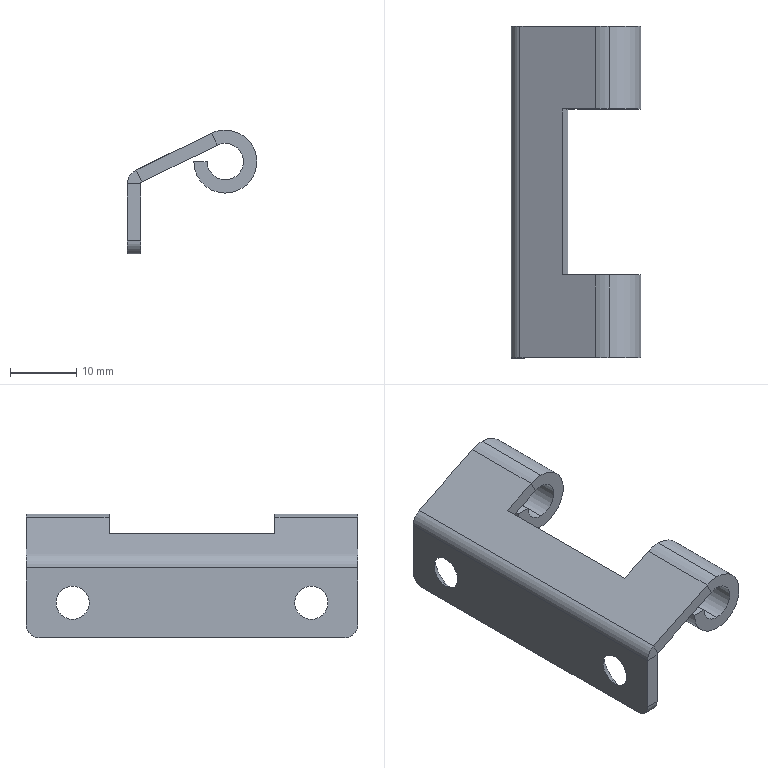Part | SolidWorks | features Cut 2, Chamfer 1, Fillet 1, FlatPattern 1, SMBaseFlange 1, SheetMetal 1 | 1 solid | 40 faces | box 19.5 x 50 x 18.659 mm | volume 2993 mm3 | plane 20 | cylinder 16 | cone 4 | commonest cylinder face diameters 5.5 x6 9.5 x6 4 x2 0.6 x1 4.6 x1
STEP:
#1=CARTESIAN_POINT('',(0.,43.,7.8));
#2=VERTEX_POINT('',#1);
#3=CARTESIAN_POINT('',(0.,43.,2.8));
#4=VERTEX_POINT('',#3);
#5=CARTESIAN_POINT('',(0.,43.,5.3));
#6=DIRECTION('',(1.,0.,0.));
#7=DIRECTION('',(0.,0.,-1.));
#8=AXIS2_PLACEMENT_3D('',#5,#6,#7);
#9=CIRCLE('',#8,2.5);
#10=EDGE_CURVE('',#2,#4,#9,.T.);
#11=ORIENTED_EDGE('',*,*,#10,.F.);
#12=CARTESIAN_POINT('',(2.,43.,9.8));
#13=VERTEX_POINT('',#12);
#14=CARTESIAN_POINT('',(0.,43.,7.8));
#15=DIRECTION('',(0.7071,0.,0.7071));
#16=VECTOR('',#15,1000.);
#17=LINE('',#14,#16);
#18=EDGE_CURVE('',#2,#13,#17,.T.);
#19=ORIENTED_EDGE('',*,*,#18,.T.);
#20=CARTESIAN_POINT('',(2.,43.,0.8));
#21=VERTEX_POINT('',#20);
#22=CARTESIAN_POINT('',(2.,43.,5.3));
#23=DIRECTION('',(-1.,0.,0.));
#24=DIRECTION('',(0.,0.,-1.));
#25=AXIS2_PLACEMENT_3D('',#22,#23,#24);
#26=CIRCLE('',#25,4.5);
#27=EDGE_CURVE('',#21,#13,#26,.T.);
#28=ORIENTED_EDGE('',*,*,#27,.F.);
#29=CARTESIAN_POINT('',(0.,43.,2.8));
#30=DIRECTION('',(0.7071,0.,-0.7071));
#31=VECTOR('',#30,1000.);
#32=LINE('',#29,#31);
#33=EDGE_CURVE('',#4,#21,#32,.T.);
#34=ORIENTED_EDGE('',*,*,#33,.F.);
#35=EDGE_LOOP('',(#11,#19,#28,#34));
#36=FACE_OUTER_BOUND('',#35,.T.);
#37=CARTESIAN_POINT('',(0.,43.,5.3));
#38=DIRECTION('',(1.,0.,0.));
#39=DIRECTION('',(0.,0.,-1.));
#40=AXIS2_PLACEMENT_3D('',#37,#38,#39);
#41=CONICAL_SURFACE('',#40,2.5,0.7854);
#42=ADVANCED_FACE('',(#36),#41,.F.);
#43=CARTESIAN_POINT('',(0.,7.,7.8));
#44=VERTEX_POINT('',#43);
#45=CARTESIAN_POINT('',(0.,7.,2.8));
#46=VERTEX_POINT('',#45);
#47=CARTESIAN_POINT('',(0.,7.,5.3));
#48=DIRECTION('',(1.,0.,0.));
#49=DIRECTION('',(0.,0.,-1.));
#50=AXIS2_PLACEMENT_3D('',#47,#48,#49);
#51=CIRCLE('',#50,2.5);
#52=EDGE_CURVE('',#44,#46,#51,.T.);
#53=ORIENTED_EDGE('',*,*,#52,.F.);
#54=CARTESIAN_POINT('',(2.,7.,9.8));
#55=VERTEX_POINT('',#54);
#56=CARTESIAN_POINT('',(0.,7.,7.8));
#57=DIRECTION('',(0.7071,0.,0.7071));
#58=VECTOR('',#57,1000.);
#59=LINE('',#56,#58);
#60=EDGE_CURVE('',#44,#55,#59,.T.);
#61=ORIENTED_EDGE('',*,*,#60,.T.);
#62=CARTESIAN_POINT('',(2.,7.,0.8));
#63=VERTEX_POINT('',#62);
#64=CARTESIAN_POINT('',(2.,7.,5.3));
#65=DIRECTION('',(-1.,0.,0.));
#66=DIRECTION('',(0.,0.,-1.));
#67=AXIS2_PLACEMENT_3D('',#64,#65,#66);
#68=CIRCLE('',#67,4.5);
#69=EDGE_CURVE('',#63,#55,#68,.T.);
#70=ORIENTED_EDGE('',*,*,#69,.F.);
#71=CARTESIAN_POINT('',(0.,7.,2.8));
#72=DIRECTION('',(0.7071,0.,-0.7071));
#73=VECTOR('',#72,1000.);
#74=LINE('',#71,#73);
#75=EDGE_CURVE('',#46,#63,#74,.T.);
#76=ORIENTED_EDGE('',*,*,#75,.F.);
#77=EDGE_LOOP('',(#53,#61,#70,#76));
#78=FACE_OUTER_BOUND('',#77,.T.);
#79=CARTESIAN_POINT('',(0.,7.,5.3));
#80=DIRECTION('',(1.,0.,0.));
#81=DIRECTION('',(0.,0.,-1.));
#82=AXIS2_PLACEMENT_3D('',#79,#80,#81);
#83=CONICAL_SURFACE('',#82,2.5,0.7854);
#84=ADVANCED_FACE('',(#78),#83,.F.);
#85=CARTESIAN_POINT('',(14.75,12.5,16.659));
#86=VERTEX_POINT('',#85);
#87=CARTESIAN_POINT('',(13.544,12.5,16.381));
#88=VERTEX_POINT('',#87);
#89=CARTESIAN_POINT('',(14.75,12.5,13.909));
#90=DIRECTION('',(0.,-1.,0.));
#91=DIRECTION('',(1.,0.,0.));
#92=AXIS2_PLACEMENT_3D('',#89,#90,#91);
#93=CIRCLE('',#92,2.75);
#94=EDGE_CURVE('',#86,#88,#93,.T.);
#95=ORIENTED_EDGE('',*,*,#94,.F.);
#96=CARTESIAN_POINT('',(14.75,0.,16.659));
#97=VERTEX_POINT('',#96);
#98=CARTESIAN_POINT('',(14.75,50.,16.659));
#99=DIRECTION('',(0.,-1.,0.));
#100=VECTOR('',#99,1000.);
#101=LINE('',#98,#100);
#102=EDGE_CURVE('',#86,#97,#101,.T.);
#103=ORIENTED_EDGE('',*,*,#102,.T.);
#104=CARTESIAN_POINT('',(13.544,0.,16.381));
#105=VERTEX_POINT('',#104);
#106=CARTESIAN_POINT('',(14.75,0.,13.909));
#107=DIRECTION('',(0.,1.,0.));
#108=DIRECTION('',(1.,0.,0.));
#109=AXIS2_PLACEMENT_3D('',#106,#107,#108);
#110=CIRCLE('',#109,2.75);
#111=EDGE_CURVE('',#105,#97,#110,.T.);
#112=ORIENTED_EDGE('',*,*,#111,.F.);
#113=CARTESIAN_POINT('',(13.544,50.,16.381));
#114=DIRECTION('',(0.,-1.,0.));
#115=VECTOR('',#114,1000.);
#116=LINE('',#113,#115);
#117=EDGE_CURVE('',#88,#105,#116,.T.);
#118=ORIENTED_EDGE('',*,*,#117,.F.);
#119=EDGE_LOOP('',(#95,#103,#112,#118));
#120=FACE_OUTER_BOUND('',#119,.T.);
#121=CARTESIAN_POINT('',(14.75,50.,13.909));
#122=DIRECTION('',(0.,-1.,0.));
#123=DIRECTION('',(0.,0.,-1.));
#124=AXIS2_PLACEMENT_3D('',#121,#122,#123);
#125=CYLINDRICAL_SURFACE('',#124,2.75);
#126=ADVANCED_FACE('',(#120),#125,.F.);
#127=ORIENTED_EDGE('',*,*,#102,.F.);
#128=CARTESIAN_POINT('',(14.75,12.5,11.159));
#129=VERTEX_POINT('',#128);
#130=CARTESIAN_POINT('',(14.75,12.5,13.909));
#131=DIRECTION('',(0.,-1.,0.));
#132=DIRECTION('',(1.,0.,0.));
#133=AXIS2_PLACEMENT_3D('',#130,#131,#132);
#134=CIRCLE('',#133,2.75);
#135=EDGE_CURVE('',#129,#86,#134,.T.);
#136=ORIENTED_EDGE('',*,*,#135,.F.);
#137=CARTESIAN_POINT('',(14.75,0.,11.159));
#138=VERTEX_POINT('',#137);
#139=CARTESIAN_POINT('',(14.75,50.,11.159));
#140=DIRECTION('',(0.,-1.,0.));
#141=VECTOR('',#140,1000.);
#142=LINE('',#139,#141);
#143=EDGE_CURVE('',#129,#138,#142,.T.);
#144=ORIENTED_EDGE('',*,*,#143,.T.);
#145=CARTESIAN_POINT('',(14.75,0.,13.909));
#146=DIRECTION('',(0.,1.,0.));
#147=DIRECTION('',(1.,0.,0.));
#148=AXIS2_PLACEMENT_3D('',#145,#146,#147);
#149=CIRCLE('',#148,2.75);
#150=EDGE_CURVE('',#97,#138,#149,.T.);
#151=ORIENTED_EDGE('',*,*,#150,.F.);
#152=EDGE_LOOP('',(#127,#136,#144,#151));
#153=FACE_OUTER_BOUND('',#152,.T.);
#154=CARTESIAN_POINT('',(14.75,50.,13.909));
#155=DIRECTION('',(0.,-1.,0.));
#156=DIRECTION('',(0.,0.,-1.));
#157=AXIS2_PLACEMENT_3D('',#154,#155,#156);
#158=CYLINDRICAL_SURFACE('',#157,2.75);
#159=ADVANCED_FACE('',(#153),#158,.F.);
#160=CARTESIAN_POINT('',(13.544,50.,16.381));
#161=VERTEX_POINT('',#160);
#162=CARTESIAN_POINT('',(14.75,50.,16.659));
#163=VERTEX_POINT('',#162);
#164=CARTESIAN_POINT('',(14.75,50.,13.909));
#165=DIRECTION('',(0.,1.,0.));
#166=DIRECTION('',(1.,0.,0.));
#167=AXIS2_PLACEMENT_3D('',#164,#165,#166);
#168=CIRCLE('',#167,2.75);
#169=EDGE_CURVE('',#161,#163,#168,.T.);
#170=ORIENTED_EDGE('',*,*,#169,.T.);
#171=CARTESIAN_POINT('',(14.75,37.5,16.659));
#172=VERTEX_POINT('',#171);
#173=CARTESIAN_POINT('',(14.75,50.,16.659));
#174=DIRECTION('',(0.,-1.,0.));
#175=VECTOR('',#174,1000.);
#176=LINE('',#173,#175);
#177=EDGE_CURVE('',#163,#172,#176,.T.);
#178=ORIENTED_EDGE('',*,*,#177,.T.);
#179=CARTESIAN_POINT('',(13.544,37.5,16.381));
#180=VERTEX_POINT('',#179);
#181=CARTESIAN_POINT('',(14.75,37.5,13.909));
#182=DIRECTION('',(0.,1.,0.));
#183=DIRECTION('',(0.,0.,1.));
#184=AXIS2_PLACEMENT_3D('',#181,#182,#183);
#185=CIRCLE('',#184,2.75);
#186=EDGE_CURVE('',#180,#172,#185,.T.);
#187=ORIENTED_EDGE('',*,*,#186,.F.);
#188=CARTESIAN_POINT('',(13.544,50.,16.381));
#189=DIRECTION('',(0.,-1.,0.));
#190=VECTOR('',#189,1000.);
#191=LINE('',#188,#190);
#192=EDGE_CURVE('',#161,#180,#191,.T.);
#193=ORIENTED_EDGE('',*,*,#192,.F.);
#194=EDGE_LOOP('',(#170,#178,#187,#193));
#195=FACE_OUTER_BOUND('',#194,.T.);
#196=CARTESIAN_POINT('',(14.75,50.,13.909));
#197=DIRECTION('',(0.,-1.,0.));
#198=DIRECTION('',(0.,0.,-1.));
#199=AXIS2_PLACEMENT_3D('',#196,#197,#198);
#200=CYLINDRICAL_SURFACE('',#199,2.75);
#201=ADVANCED_FACE('',(#195),#200,.F.);
#202=ORIENTED_EDGE('',*,*,#177,.F.);
#203=CARTESIAN_POINT('',(14.75,50.,11.159));
#204=VERTEX_POINT('',#203);
#205=CARTESIAN_POINT('',(14.75,50.,13.909));
#206=DIRECTION('',(0.,1.,0.));
#207=DIRECTION('',(1.,0.,0.));
#208=AXIS2_PLACEMENT_3D('',#205,#206,#207);
#209=CIRCLE('',#208,2.75);
#210=EDGE_CURVE('',#163,#204,#209,.T.);
#211=ORIENTED_EDGE('',*,*,#210,.T.);
#212=CARTESIAN_POINT('',(14.75,37.5,11.159));
#213=VERTEX_POINT('',#212);
#214=CARTESIAN_POINT('',(14.75,50.,11.159));
#215=DIRECTION('',(0.,-1.,0.));
#216=VECTOR('',#215,1000.);
#217=LINE('',#214,#216);
#218=EDGE_CURVE('',#204,#213,#217,.T.);
#219=ORIENTED_EDGE('',*,*,#218,.T.);
#220=CARTESIAN_POINT('',(14.75,37.5,13.909));
#221=DIRECTION('',(0.,1.,0.));
#222=DIRECTION('',(0.,0.,1.));
#223=AXIS2_PLACEMENT_3D('',#220,#221,#222);
#224=CIRCLE('',#223,2.75);
#225=EDGE_CURVE('',#172,#213,#224,.T.);
#226=ORIENTED_EDGE('',*,*,#225,.F.);
#227=EDGE_LOOP('',(#202,#211,#219,#226));
#228=FACE_OUTER_BOUND('',#227,.T.);
#229=CARTESIAN_POINT('',(14.75,50.,13.909));
#230=DIRECTION('',(0.,-1.,0.));
#231=DIRECTION('',(0.,0.,-1.));
#232=AXIS2_PLACEMENT_3D('',#229,#230,#231);
#233=CYLINDRICAL_SURFACE('',#232,2.75);
#234=ADVANCED_FACE('',(#228),#233,.F.);
#235=CARTESIAN_POINT('',(14.75,12.5,9.159));
#236=VERTEX_POINT('',#235);
#237=CARTESIAN_POINT('',(14.75,12.5,18.659));
#238=VERTEX_POINT('',#237);
#239=CARTESIAN_POINT('',(14.75,12.5,13.909));
#240=DIRECTION('',(0.,-1.,0.));
#241=DIRECTION('',(0.,0.,-1.));
#242=AXIS2_PLACEMENT_3D('',#239,#240,#241);
#243=CIRCLE('',#242,4.75);
#244=EDGE_CURVE('',#236,#238,#243,.T.);
#245=ORIENTED_EDGE('',*,*,#244,.T.);
#246=CARTESIAN_POINT('',(14.75,0.,18.659));
#247=VERTEX_POINT('',#246);
#248=CARTESIAN_POINT('',(14.75,50.,18.659));
#249=DIRECTION('',(0.,-1.,0.));
#250=VECTOR('',#249,1000.);
#251=LINE('',#248,#250);
#252=EDGE_CURVE('',#238,#247,#251,.T.);
#253=ORIENTED_EDGE('',*,*,#252,.T.);
#254=CARTESIAN_POINT('',(14.75,0.,9.159));
#255=VERTEX_POINT('',#254);
#256=CARTESIAN_POINT('',(14.75,0.,13.909));
#257=DIRECTION('',(0.,1.,0.));
#258=DIRECTION('',(0.,0.,1.));
#259=AXIS2_PLACEMENT_3D('',#256,#257,#258);
#260=CIRCLE('',#259,4.75);
#261=EDGE_CURVE('',#247,#255,#260,.T.);
#262=ORIENTED_EDGE('',*,*,#261,.T.);
#263=CARTESIAN_POINT('',(14.75,50.,9.159));
#264=DIRECTION('',(0.,-1.,0.));
#265=VECTOR('',#264,1000.);
#266=LINE('',#263,#265);
#267=EDGE_CURVE('',#236,#255,#266,.T.);
#268=ORIENTED_EDGE('',*,*,#267,.F.);
#269=EDGE_LOOP('',(#245,#253,#262,#268));
#270=FACE_OUTER_BOUND('',#269,.T.);
#271=CARTESIAN_POINT('',(14.75,50.,13.909));
#272=DIRECTION('',(0.,-1.,0.));
#273=DIRECTION('',(0.,0.,-1.));
#274=AXIS2_PLACEMENT_3D('',#271,#272,#273);
#275=CYLINDRICAL_SURFACE('',#274,4.75);
#276=ADVANCED_FACE('',(#270),#275,.T.);
#277=CARTESIAN_POINT('',(10.,12.5,13.903));
#278=VERTEX_POINT('',#277);
#279=CARTESIAN_POINT('',(14.75,12.5,13.909));
#280=DIRECTION('',(0.,-1.,0.));
#281=DIRECTION('',(0.,0.,-1.));
#282=AXIS2_PLACEMENT_3D('',#279,#280,#281);
#283=CIRCLE('',#282,4.75);
#284=EDGE_CURVE('',#278,#236,#283,.T.);
#285=ORIENTED_EDGE('',*,*,#284,.T.);
#286=ORIENTED_EDGE('',*,*,#267,.T.);
#287=CARTESIAN_POINT('',(10.,0.,13.903));
#288=VERTEX_POINT('',#287);
#289=CARTESIAN_POINT('',(14.75,0.,13.909));
#290=DIRECTION('',(0.,1.,0.));
#291=DIRECTION('',(0.,0.,1.));
#292=AXIS2_PLACEMENT_3D('',#289,#290,#291);
#293=CIRCLE('',#292,4.75);
#294=EDGE_CURVE('',#255,#288,#293,.T.);
#295=ORIENTED_EDGE('',*,*,#294,.T.);
#296=CARTESIAN_POINT('',(10.,50.,13.903));
#297=DIRECTION('',(0.,-1.,0.));
#298=VECTOR('',#297,1000.);
#299=LINE('',#296,#298);
#300=EDGE_CURVE('',#278,#288,#299,.T.);
#301=ORIENTED_EDGE('',*,*,#300,.F.);
#302=EDGE_LOOP('',(#285,#286,#295,#301));
#303=FACE_OUTER_BOUND('',#302,.T.);
#304=CARTESIAN_POINT('',(14.75,50.,13.909));
#305=DIRECTION('',(0.,-1.,0.));
#306=DIRECTION('',(0.,0.,-1.));
#307=AXIS2_PLACEMENT_3D('',#304,#305,#306);
#308=CYLINDRICAL_SURFACE('',#307,4.75);
#309=ADVANCED_FACE('',(#303),#308,.T.);
#310=CARTESIAN_POINT('',(14.75,50.,18.659));
#311=VERTEX_POINT('',#310);
#312=CARTESIAN_POINT('',(14.75,50.,9.159));
#313=VERTEX_POINT('',#312);
#314=CARTESIAN_POINT('',(14.75,50.,13.909));
#315=DIRECTION('',(0.,1.,0.));
#316=DIRECTION('',(0.,0.,1.));
#317=AXIS2_PLACEMENT_3D('',#314,#315,#316);
#318=CIRCLE('',#317,4.75);
#319=EDGE_CURVE('',#311,#313,#318,.T.);
#320=ORIENTED_EDGE('',*,*,#319,.F.);
#321=CARTESIAN_POINT('',(14.75,37.5,18.659));
#322=VERTEX_POINT('',#321);
#323=CARTESIAN_POINT('',(14.75,50.,18.659));
#324=DIRECTION('',(0.,-1.,0.));
#325=VECTOR('',#324,1000.);
#326=LINE('',#323,#325);
#327=EDGE_CURVE('',#311,#322,#326,.T.);
#328=ORIENTED_EDGE('',*,*,#327,.T.);
#329=CARTESIAN_POINT('',(14.75,37.5,9.159));
#330=VERTEX_POINT('',#329);
#331=CARTESIAN_POINT('',(14.75,37.5,13.909));
#332=DIRECTION('',(0.,1.,0.));
#333=DIRECTION('',(0.,0.,-1.));
#334=AXIS2_PLACEMENT_3D('',#331,#332,#333);
#335=CIRCLE('',#334,4.75);
#336=EDGE_CURVE('',#322,#330,#335,.T.);
#337=ORIENTED_EDGE('',*,*,#336,.T.);
#338=CARTESIAN_POINT('',(14.75,50.,9.159));
#339=DIRECTION('',(0.,-1.,0.));
#340=VECTOR('',#339,1000.);
#341=LINE('',#338,#340);
#342=EDGE_CURVE('',#313,#330,#341,.T.);
#343=ORIENTED_EDGE('',*,*,#342,.F.);
#344=EDGE_LOOP('',(#320,#328,#337,#343));
#345=FACE_OUTER_BOUND('',#344,.T.);
#346=CARTESIAN_POINT('',(14.75,50.,13.909));
#347=DIRECTION('',(0.,-1.,0.));
#348=DIRECTION('',(0.,0.,-1.));
#349=AXIS2_PLACEMENT_3D('',#346,#347,#348);
#350=CYLINDRICAL_SURFACE('',#349,4.75);
#351=ADVANCED_FACE('',(#345),#350,.T.);
#352=CARTESIAN_POINT('',(10.,50.,13.903));
#353=VERTEX_POINT('',#352);
#354=CARTESIAN_POINT('',(14.75,50.,13.909));
#355=DIRECTION('',(0.,1.,0.));
#356=DIRECTION('',(0.,0.,1.));
#357=AXIS2_PLACEMENT_3D('',#354,#355,#356);
#358=CIRCLE('',#357,4.75);
#359=EDGE_CURVE('',#313,#353,#358,.T.);
#360=ORIENTED_EDGE('',*,*,#359,.F.);
#361=ORIENTED_EDGE('',*,*,#342,.T.);
#362=CARTESIAN_POINT('',(10.,37.5,13.903));
#363=VERTEX_POINT('',#362);
#364=CARTESIAN_POINT('',(14.75,37.5,13.909));
#365=DIRECTION('',(0.,1.,0.));
#366=DIRECTION('',(0.,0.,-1.));
#367=AXIS2_PLACEMENT_3D('',#364,#365,#366);
#368=CIRCLE('',#367,4.75);
#369=EDGE_CURVE('',#330,#363,#368,.T.);
#370=ORIENTED_EDGE('',*,*,#369,.T.);
#371=CARTESIAN_POINT('',(10.,50.,13.903));
#372=DIRECTION('',(0.,-1.,0.));
#373=VECTOR('',#372,1000.);
#374=LINE('',#371,#373);
#375=EDGE_CURVE('',#353,#363,#374,.T.);
#376=ORIENTED_EDGE('',*,*,#375,.F.);
#377=EDGE_LOOP('',(#360,#361,#370,#376));
#378=FACE_OUTER_BOUND('',#377,.T.);
#379=CARTESIAN_POINT('',(14.75,50.,13.909));
#380=DIRECTION('',(0.,-1.,0.));
#381=DIRECTION('',(0.,0.,-1.));
#382=AXIS2_PLACEMENT_3D('',#379,#380,#381);
#383=CYLINDRICAL_SURFACE('',#382,4.75);
#384=ADVANCED_FACE('',(#378),#383,.T.);
#385=ORIENTED_EDGE('',*,*,#327,.F.);
#386=CARTESIAN_POINT('',(12.668,50.,18.178));
#387=VERTEX_POINT('',#386);
#388=CARTESIAN_POINT('',(14.75,50.,13.909));
#389=DIRECTION('',(0.,1.,0.));
#390=DIRECTION('',(0.,0.,1.));
#391=AXIS2_PLACEMENT_3D('',#388,#389,#390);
#392=CIRCLE('',#391,4.75);
#393=EDGE_CURVE('',#387,#311,#392,.T.);
#394=ORIENTED_EDGE('',*,*,#393,.F.);
#395=CARTESIAN_POINT('',(12.668,37.5,18.178));
#396=VERTEX_POINT('',#395);
#397=CARTESIAN_POINT('',(12.668,50.,18.178));
#398=DIRECTION('',(0.,-1.,0.));
#399=VECTOR('',#398,1000.);
#400=LINE('',#397,#399);
#401=EDGE_CURVE('',#387,#396,#400,.T.);
#402=ORIENTED_EDGE('',*,*,#401,.T.);
#403=CARTESIAN_POINT('',(14.75,37.5,13.909));
#404=DIRECTION('',(0.,1.,0.));
#405=DIRECTION('',(0.,0.,-1.));
#406=AXIS2_PLACEMENT_3D('',#403,#404,#405);
#407=CIRCLE('',#406,4.75);
#408=EDGE_CURVE('',#396,#322,#407,.T.);
#409=ORIENTED_EDGE('',*,*,#408,.T.);
#410=EDGE_LOOP('',(#385,#394,#402,#409));
#411=FACE_OUTER_BOUND('',#410,.T.);
#412=CARTESIAN_POINT('',(14.75,50.,13.909));
#413=DIRECTION('',(0.,-1.,0.));
#414=DIRECTION('',(0.,0.,-1.));
#415=AXIS2_PLACEMENT_3D('',#412,#413,#414);
#416=CYLINDRICAL_SURFACE('',#415,4.75);
#417=ADVANCED_FACE('',(#411),#416,.T.);
#418=ORIENTED_EDGE('',*,*,#252,.F.);
#419=CARTESIAN_POINT('',(12.668,12.5,18.178));
#420=VERTEX_POINT('',#419);
#421=CARTESIAN_POINT('',(14.75,12.5,13.909));
#422=DIRECTION('',(0.,-1.,0.));
#423=DIRECTION('',(0.,0.,-1.));
#424=AXIS2_PLACEMENT_3D('',#421,#422,#423);
#425=CIRCLE('',#424,4.75);
#426=EDGE_CURVE('',#238,#420,#425,.T.);
#427=ORIENTED_EDGE('',*,*,#426,.T.);
#428=CARTESIAN_POINT('',(12.668,0.,18.178));
#429=VERTEX_POINT('',#428);
#430=CARTESIAN_POINT('',(12.668,50.,18.178));
#431=DIRECTION('',(0.,-1.,0.));
#432=VECTOR('',#431,1000.);
#433=LINE('',#430,#432);
#434=EDGE_CURVE('',#420,#429,#433,.T.);
#435=ORIENTED_EDGE('',*,*,#434,.T.);
#436=CARTESIAN_POINT('',(14.75,0.,13.909));
#437=DIRECTION('',(0.,1.,0.));
#438=DIRECTION('',(0.,0.,1.));
#439=AXIS2_PLACEMENT_3D('',#436,#437,#438);
#440=CIRCLE('',#439,4.75);
#441=EDGE_CURVE('',#429,#247,#440,.T.);
#442=ORIENTED_EDGE('',*,*,#441,.T.);
#443=EDGE_LOOP('',(#418,#427,#435,#442));
#444=FACE_OUTER_BOUND('',#443,.T.);
#445=CARTESIAN_POINT('',(14.75,50.,13.909));
#446=DIRECTION('',(0.,-1.,0.));
#447=DIRECTION('',(0.,0.,-1.));
#448=AXIS2_PLACEMENT_3D('',#445,#446,#447);
#449=CYLINDRICAL_SURFACE('',#448,4.75);
#450=ADVANCED_FACE('',(#444),#449,.T.);
#451=ORIENTED_EDGE('',*,*,#375,.T.);
#452=CARTESIAN_POINT('',(12.,37.5,13.906));
#453=VERTEX_POINT('',#452);
#454=CARTESIAN_POINT('',(12.,37.5,13.906));
#455=DIRECTION('',(-1.,0.,-0.001333));
#456=VECTOR('',#455,1000.);
#457=LINE('',#454,#456);
#458=EDGE_CURVE('',#453,#363,#457,.T.);
#459=ORIENTED_EDGE('',*,*,#458,.F.);
#460=CARTESIAN_POINT('',(12.,50.,13.906));
#461=VERTEX_POINT('',#460);
#462=CARTESIAN_POINT('',(12.,50.,13.906));
#463=DIRECTION('',(0.,-1.,0.));
#464=VECTOR('',#463,1000.);
#465=LINE('',#462,#464);
#466=EDGE_CURVE('',#461,#453,#465,.T.);
#467=ORIENTED_EDGE('',*,*,#466,.F.);
#468=CARTESIAN_POINT('',(12.,50.,13.906));
#469=DIRECTION('',(-1.,0.,-0.001333));
#470=VECTOR('',#469,1000.);
#471=LINE('',#468,#470);
#472=EDGE_CURVE('',#461,#353,#471,.T.);
#473=ORIENTED_EDGE('',*,*,#472,.T.);
#474=EDGE_LOOP('',(#451,#459,#467,#473));
#475=FACE_OUTER_BOUND('',#474,.T.);
#476=CARTESIAN_POINT('',(12.,50.,13.906));
#477=DIRECTION('',(-0.001333,0.,1.));
#478=DIRECTION('',(1.,0.,0.001333));
#479=AXIS2_PLACEMENT_3D('',#476,#477,#478);
#480=PLANE('',#479);
#481=ADVANCED_FACE('',(#475),#480,.T.);
#482=CARTESIAN_POINT('',(12.,12.5,13.906));
#483=VERTEX_POINT('',#482);
#484=CARTESIAN_POINT('',(12.,0.,13.906));
#485=VERTEX_POINT('',#484);
#486=CARTESIAN_POINT('',(12.,50.,13.906));
#487=DIRECTION('',(0.,-1.,0.));
#488=VECTOR('',#487,1000.);
#489=LINE('',#486,#488);
#490=EDGE_CURVE('',#483,#485,#489,.T.);
#491=ORIENTED_EDGE('',*,*,#490,.F.);
#492=CARTESIAN_POINT('',(12.,12.5,13.906));
#493=DIRECTION('',(-1.,0.,-0.001333));
#494=VECTOR('',#493,1000.);
#495=LINE('',#492,#494);
#496=EDGE_CURVE('',#483,#278,#495,.T.);
#497=ORIENTED_EDGE('',*,*,#496,.T.);
#498=ORIENTED_EDGE('',*,*,#300,.T.);
#499=CARTESIAN_POINT('',(12.,0.,13.906));
#500=DIRECTION('',(-1.,0.,-0.001333));
#501=VECTOR('',#500,1000.);
#502=LINE('',#499,#501);
#503=EDGE_CURVE('',#485,#288,#502,.T.);
#504=ORIENTED_EDGE('',*,*,#503,.F.);
#505=EDGE_LOOP('',(#491,#497,#498,#504));
#506=FACE_OUTER_BOUND('',#505,.T.);
#507=CARTESIAN_POINT('',(12.,50.,13.906));
#508=DIRECTION('',(-0.001333,0.,1.));
#509=DIRECTION('',(1.,0.,0.001333));
#510=AXIS2_PLACEMENT_3D('',#507,#508,#509);
#511=PLANE('',#510);
#512=ADVANCED_FACE('',(#506),#511,.T.);
#513=ORIENTED_EDGE('',*,*,#218,.F.);
#514=CARTESIAN_POINT('',(14.75,50.,13.909));
#515=DIRECTION('',(0.,1.,0.));
#516=DIRECTION('',(1.,0.,0.));
#517=AXIS2_PLACEMENT_3D('',#514,#515,#516);
#518=CIRCLE('',#517,2.75);
#519=EDGE_CURVE('',#204,#461,#518,.T.);
#520=ORIENTED_EDGE('',*,*,#519,.T.);
#521=ORIENTED_EDGE('',*,*,#466,.T.);
#522=CARTESIAN_POINT('',(14.75,37.5,13.909));
#523=DIRECTION('',(0.,1.,0.));
#524=DIRECTION('',(0.,0.,1.));
#525=AXIS2_PLACEMENT_3D('',#522,#523,#524);
#526=CIRCLE('',#525,2.75);
#527=EDGE_CURVE('',#213,#453,#526,.T.);
#528=ORIENTED_EDGE('',*,*,#527,.F.);
#529=EDGE_LOOP('',(#513,#520,#521,#528));
#530=FACE_OUTER_BOUND('',#529,.T.);
#531=CARTESIAN_POINT('',(14.75,50.,13.909));
#532=DIRECTION('',(0.,-1.,0.));
#533=DIRECTION('',(0.,0.,-1.));
#534=AXIS2_PLACEMENT_3D('',#531,#532,#533);
#535=CYLINDRICAL_SURFACE('',#534,2.75);
#536=ADVANCED_FACE('',(#530),#535,.F.);
#537=ORIENTED_EDGE('',*,*,#143,.F.);
#538=CARTESIAN_POINT('',(14.75,12.5,13.909));
#539=DIRECTION('',(0.,-1.,0.));
#540=DIRECTION('',(1.,0.,0.));
#541=AXIS2_PLACEMENT_3D('',#538,#539,#540);
#542=CIRCLE('',#541,2.75);
#543=EDGE_CURVE('',#483,#129,#542,.T.);
#544=ORIENTED_EDGE('',*,*,#543,.F.);
#545=ORIENTED_EDGE('',*,*,#490,.T.);
#546=CARTESIAN_POINT('',(14.75,0.,13.909));
#547=DIRECTION('',(0.,1.,0.));
#548=DIRECTION('',(1.,0.,0.));
#549=AXIS2_PLACEMENT_3D('',#546,#547,#548);
#550=CIRCLE('',#549,2.75);
#551=EDGE_CURVE('',#138,#485,#550,.T.);
#552=ORIENTED_EDGE('',*,*,#551,.F.);
#553=EDGE_LOOP('',(#537,#544,#545,#552));
#554=FACE_OUTER_BOUND('',#553,.T.);
#555=CARTESIAN_POINT('',(14.75,50.,13.909));
#556=DIRECTION('',(0.,-1.,0.));
#557=DIRECTION('',(0.,0.,-1.));
#558=AXIS2_PLACEMENT_3D('',#555,#556,#557);
#559=CYLINDRICAL_SURFACE('',#558,2.75);
#560=ADVANCED_FACE('',(#554),#559,.F.);
#561=ORIENTED_EDGE('',*,*,#192,.T.);
#562=CARTESIAN_POINT('',(8.5,37.5,13.921));
#563=VERTEX_POINT('',#562);
#564=CARTESIAN_POINT('',(0.8767,37.5,10.202));
#565=DIRECTION('',(0.8988,0.,0.4384));
#566=VECTOR('',#565,1000.);
#567=LINE('',#564,#566);
#568=EDGE_CURVE('',#563,#180,#567,.T.);
#569=ORIENTED_EDGE('',*,*,#568,.F.);
#570=CARTESIAN_POINT('',(8.5,12.5,13.921));
#571=VERTEX_POINT('',#570);
#572=CARTESIAN_POINT('',(8.5,50.,13.921));
#573=DIRECTION('',(0.,1.,0.));
#574=VECTOR('',#573,1000.);
#575=LINE('',#572,#574);
#576=EDGE_CURVE('',#571,#563,#575,.T.);
#577=ORIENTED_EDGE('',*,*,#576,.F.);
#578=CARTESIAN_POINT('',(0.8767,12.5,10.202));
#579=DIRECTION('',(-0.8988,0.,-0.4384));
#580=VECTOR('',#579,1000.);
#581=LINE('',#578,#580);
#582=EDGE_CURVE('',#88,#571,#581,.T.);
#583=ORIENTED_EDGE('',*,*,#582,.F.);
#584=ORIENTED_EDGE('',*,*,#117,.T.);
#585=CARTESIAN_POINT('',(2.168,0.,10.832));
#586=VERTEX_POINT('',#585);
#587=CARTESIAN_POINT('',(0.8767,0.,10.202));
#588=DIRECTION('',(0.8988,0.,0.4384));
#589=VECTOR('',#588,1000.);
#590=LINE('',#587,#589);
#591=EDGE_CURVE('',#586,#105,#590,.T.);
#592=ORIENTED_EDGE('',*,*,#591,.F.);
#593=CARTESIAN_POINT('',(2.168,50.,10.832));
#594=VERTEX_POINT('',#593);
#595=CARTESIAN_POINT('',(2.168,50.,10.832));
#596=DIRECTION('',(0.,-1.,0.));
#597=VECTOR('',#596,1000.);
#598=LINE('',#595,#597);
#599=EDGE_CURVE('',#594,#586,#598,.T.);
#600=ORIENTED_EDGE('',*,*,#599,.F.);
#601=CARTESIAN_POINT('',(0.8767,50.,10.202));
#602=DIRECTION('',(0.8988,0.,0.4384));
#603=VECTOR('',#602,1000.);
#604=LINE('',#601,#603);
#605=EDGE_CURVE('',#594,#161,#604,.T.);
#606=ORIENTED_EDGE('',*,*,#605,.T.);
#607=EDGE_LOOP('',(#561,#569,#577,#583,#584,#592,#600,#606));
#608=FACE_OUTER_BOUND('',#607,.T.);
#609=CARTESIAN_POINT('',(0.8767,50.,10.202));
#610=DIRECTION('',(0.4384,0.,-0.8988));
#611=DIRECTION('',(-0.8988,0.,-0.4384));
#612=AXIS2_PLACEMENT_3D('',#609,#610,#611);
#613=PLANE('',#612);
#614=ADVANCED_FACE('',(#608),#613,.T.);
#615=CARTESIAN_POINT('',(7.623,37.5,15.718));
#616=VERTEX_POINT('',#615);
#617=CARTESIAN_POINT('',(0.,37.5,12.));
#618=DIRECTION('',(0.8988,0.,0.4384));
#619=VECTOR('',#618,1000.);
#620=LINE('',#617,#619);
#621=EDGE_CURVE('',#616,#396,#620,.T.);
#622=ORIENTED_EDGE('',*,*,#621,.T.);
#623=ORIENTED_EDGE('',*,*,#401,.F.);
#624=CARTESIAN_POINT('',(1.292,50.,12.63));
#625=VERTEX_POINT('',#624);
#626=CARTESIAN_POINT('',(0.,50.,12.));
#627=DIRECTION('',(0.8988,0.,0.4384));
#628=VECTOR('',#627,1000.);
#629=LINE('',#626,#628);
#630=EDGE_CURVE('',#625,#387,#629,.T.);
#631=ORIENTED_EDGE('',*,*,#630,.F.);
#632=CARTESIAN_POINT('',(1.292,0.,12.63));
#633=VERTEX_POINT('',#632);
#634=CARTESIAN_POINT('',(1.292,50.,12.63));
#635=DIRECTION('',(0.,-1.,0.));
#636=VECTOR('',#635,1000.);
#637=LINE('',#634,#636);
#638=EDGE_CURVE('',#625,#633,#637,.T.);
#639=ORIENTED_EDGE('',*,*,#638,.T.);
#640=CARTESIAN_POINT('',(0.,0.,12.));
#641=DIRECTION('',(0.8988,0.,0.4384));
#642=VECTOR('',#641,1000.);
#643=LINE('',#640,#642);
#644=EDGE_CURVE('',#633,#429,#643,.T.);
#645=ORIENTED_EDGE('',*,*,#644,.T.);
#646=ORIENTED_EDGE('',*,*,#434,.F.);
#647=CARTESIAN_POINT('',(7.623,12.5,15.718));
#648=VERTEX_POINT('',#647);
#649=CARTESIAN_POINT('',(0.,12.5,12.));
#650=DIRECTION('',(-0.8988,0.,-0.4384));
#651=VECTOR('',#650,1000.);
#652=LINE('',#649,#651);
#653=EDGE_CURVE('',#420,#648,#652,.T.);
#654=ORIENTED_EDGE('',*,*,#653,.T.);
#655=CARTESIAN_POINT('',(7.623,50.,15.718));
#656=DIRECTION('',(0.,1.,0.));
#657=VECTOR('',#656,1000.);
#658=LINE('',#655,#657);
#659=EDGE_CURVE('',#648,#616,#658,.T.);
#660=ORIENTED_EDGE('',*,*,#659,.T.);
#661=EDGE_LOOP('',(#622,#623,#631,#639,#645,#646,#654,#660));
#662=FACE_OUTER_BOUND('',#661,.T.);
#663=CARTESIAN_POINT('',(0.,50.,12.));
#664=DIRECTION('',(0.4384,0.,-0.8988));
#665=DIRECTION('',(-0.8988,0.,-0.4384));
#666=AXIS2_PLACEMENT_3D('',#663,#664,#665);
#667=PLANE('',#666);
#668=ADVANCED_FACE('',(#662),#667,.F.);
#669=CARTESIAN_POINT('',(12.668,50.,18.178));
#670=DIRECTION('',(0.4384,0.,-0.8988));
#671=VECTOR('',#670,1000.);
#672=LINE('',#669,#671);
#673=EDGE_CURVE('',#387,#161,#672,.T.);
#674=ORIENTED_EDGE('',*,*,#673,.F.);
#675=ORIENTED_EDGE('',*,*,#393,.T.);
#676=ORIENTED_EDGE('',*,*,#319,.T.);
#677=ORIENTED_EDGE('',*,*,#359,.T.);
#678=ORIENTED_EDGE('',*,*,#472,.F.);
#679=ORIENTED_EDGE('',*,*,#519,.F.);
#680=ORIENTED_EDGE('',*,*,#210,.F.);
#681=ORIENTED_EDGE('',*,*,#169,.F.);
#682=EDGE_LOOP('',(#674,#675,#676,#677,#678,#679,#680,#681));
#683=FACE_OUTER_BOUND('',#682,.T.);
#684=CARTESIAN_POINT('',(12.668,50.,18.178));
#685=DIRECTION('',(0.,1.,0.));
#686=DIRECTION('',(0.,0.,1.));
#687=AXIS2_PLACEMENT_3D('',#684,#685,#686);
#688=PLANE('',#687);
#689=ADVANCED_FACE('',(#683),#688,.T.);
#690=CARTESIAN_POINT('',(13.544,0.,16.381));
#691=DIRECTION('',(-0.4384,0.,0.8988));
#692=VECTOR('',#691,1000.);
#693=LINE('',#690,#692);
#694=EDGE_CURVE('',#105,#429,#693,.T.);
#695=ORIENTED_EDGE('',*,*,#694,.F.);
#696=ORIENTED_EDGE('',*,*,#111,.T.);
#697=ORIENTED_EDGE('',*,*,#150,.T.);
#698=ORIENTED_EDGE('',*,*,#551,.T.);
#699=ORIENTED_EDGE('',*,*,#503,.T.);
#700=ORIENTED_EDGE('',*,*,#294,.F.);
#701=ORIENTED_EDGE('',*,*,#261,.F.);
#702=ORIENTED_EDGE('',*,*,#441,.F.);
#703=EDGE_LOOP('',(#695,#696,#697,#698,#699,#700,#701,#702));
#704=FACE_OUTER_BOUND('',#703,.T.);
#705=CARTESIAN_POINT('',(13.544,0.,16.381));
#706=DIRECTION('',(0.,-1.,0.));
#707=DIRECTION('',(0.,0.,-1.));
#708=AXIS2_PLACEMENT_3D('',#705,#706,#707);
#709=PLANE('',#708);
#710=ADVANCED_FACE('',(#704),#709,.T.);
#711=CARTESIAN_POINT('',(0.,50.,10.563));
#712=VERTEX_POINT('',#711);
#713=CARTESIAN_POINT('',(2.,50.,10.563));
#714=VERTEX_POINT('',#713);
#715=CARTESIAN_POINT('',(0.,50.,10.563));
#716=DIRECTION('',(1.,0.,0.));
#717=VECTOR('',#716,1000.);
#718=LINE('',#715,#717);
#719=EDGE_CURVE('',#712,#714,#718,.T.);
#720=ORIENTED_EDGE('',*,*,#719,.F.);
#721=CARTESIAN_POINT('',(2.3,50.,10.563));
#722=DIRECTION('',(0.,1.,0.));
#723=DIRECTION('',(0.,0.,-1.));
#724=AXIS2_PLACEMENT_3D('',#721,#722,#723);
#725=CIRCLE('',#724,2.3);
#726=EDGE_CURVE('',#712,#625,#725,.T.);
#727=ORIENTED_EDGE('',*,*,#726,.T.);
#728=CARTESIAN_POINT('',(2.168,50.,10.832));
#729=DIRECTION('',(-0.4384,0.,0.8988));
#730=VECTOR('',#729,1000.);
#731=LINE('',#728,#730);
#732=EDGE_CURVE('',#594,#625,#731,.T.);
#733=ORIENTED_EDGE('',*,*,#732,.F.);
#734=CARTESIAN_POINT('',(2.3,50.,10.563));
#735=DIRECTION('',(0.,1.,0.));
#736=DIRECTION('',(1.,0.,0.));
#737=AXIS2_PLACEMENT_3D('',#734,#735,#736);
#738=CIRCLE('',#737,0.3);
#739=EDGE_CURVE('',#714,#594,#738,.T.);
#740=ORIENTED_EDGE('',*,*,#739,.F.);
#741=EDGE_LOOP('',(#720,#727,#733,#740));
#742=FACE_OUTER_BOUND('',#741,.T.);
#743=CARTESIAN_POINT('',(0.,50.,10.563));
#744=DIRECTION('',(0.,1.,0.));
#745=DIRECTION('',(0.,0.,1.));
#746=AXIS2_PLACEMENT_3D('',#743,#744,#745);
#747=PLANE('',#746);
#748=ADVANCED_FACE('',(#742),#747,.T.);
#749=CARTESIAN_POINT('',(2.,50.,2.));
#750=VERTEX_POINT('',#749);
#751=CARTESIAN_POINT('',(2.,50.,0.));
#752=DIRECTION('',(0.,0.,1.));
#753=VECTOR('',#752,1000.);
#754=LINE('',#751,#753);
#755=EDGE_CURVE('',#750,#714,#754,.T.);
#756=ORIENTED_EDGE('',*,*,#755,.F.);
#757=CARTESIAN_POINT('',(0.,50.,2.));
#758=VERTEX_POINT('',#757);
#759=CARTESIAN_POINT('',(2.168,50.,2.));
#760=DIRECTION('',(-1.,0.,0.));
#761=VECTOR('',#760,1000.);
#762=LINE('',#759,#761);
#763=EDGE_CURVE('',#750,#758,#762,.T.);
#764=ORIENTED_EDGE('',*,*,#763,.T.);
#765=CARTESIAN_POINT('',(0.,50.,0.));
#766=DIRECTION('',(0.,0.,1.));
#767=VECTOR('',#766,1000.);
#768=LINE('',#765,#767);
#769=EDGE_CURVE('',#758,#712,#768,.T.);
#770=ORIENTED_EDGE('',*,*,#769,.T.);
#771=ORIENTED_EDGE('',*,*,#719,.T.);
#772=EDGE_LOOP('',(#756,#764,#770,#771));
#773=FACE_OUTER_BOUND('',#772,.T.);
#774=CARTESIAN_POINT('',(2.168,50.,10.832));
#775=DIRECTION('',(0.,1.,0.));
#776=DIRECTION('',(0.,0.,1.));
#777=AXIS2_PLACEMENT_3D('',#774,#775,#776);
#778=PLANE('',#777);
#779=ADVANCED_FACE('',(#773),#778,.T.);
#780=CARTESIAN_POINT('',(1.292,0.,12.63));
#781=DIRECTION('',(0.4384,0.,-0.8988));
#782=VECTOR('',#781,1000.);
#783=LINE('',#780,#782);
#784=EDGE_CURVE('',#633,#586,#783,.T.);
#785=ORIENTED_EDGE('',*,*,#784,.F.);
#786=CARTESIAN_POINT('',(0.,0.,10.563));
#787=VERTEX_POINT('',#786);
#788=CARTESIAN_POINT('',(2.3,0.,10.563));
#789=DIRECTION('',(0.,1.,0.));
#790=DIRECTION('',(0.,0.,-1.));
#791=AXIS2_PLACEMENT_3D('',#788,#789,#790);
#792=CIRCLE('',#791,2.3);
#793=EDGE_CURVE('',#787,#633,#792,.T.);
#794=ORIENTED_EDGE('',*,*,#793,.F.);
#795=CARTESIAN_POINT('',(2.,0.,10.563));
#796=VERTEX_POINT('',#795);
#797=CARTESIAN_POINT('',(2.,0.,10.563));
#798=DIRECTION('',(-1.,0.,0.));
#799=VECTOR('',#798,1000.);
#800=LINE('',#797,#799);
#801=EDGE_CURVE('',#796,#787,#800,.T.);
#802=ORIENTED_EDGE('',*,*,#801,.F.);
#803=CARTESIAN_POINT('',(2.3,0.,10.563));
#804=DIRECTION('',(0.,1.,0.));
#805=DIRECTION('',(1.,0.,0.));
#806=AXIS2_PLACEMENT_3D('',#803,#804,#805);
#807=CIRCLE('',#806,0.3);
#808=EDGE_CURVE('',#796,#586,#807,.T.);
#809=ORIENTED_EDGE('',*,*,#808,.T.);
#810=EDGE_LOOP('',(#785,#794,#802,#809));
#811=FACE_OUTER_BOUND('',#810,.T.);
#812=CARTESIAN_POINT('',(1.292,0.,12.63));
#813=DIRECTION('',(0.,-1.,0.));
#814=DIRECTION('',(0.,0.,-1.));
#815=AXIS2_PLACEMENT_3D('',#812,#813,#814);
#816=PLANE('',#815);
#817=ADVANCED_FACE('',(#811),#816,.T.);
#818=ORIENTED_EDGE('',*,*,#644,.F.);
#819=ORIENTED_EDGE('',*,*,#784,.T.);
#820=ORIENTED_EDGE('',*,*,#591,.T.);
#821=ORIENTED_EDGE('',*,*,#694,.T.);
#822=EDGE_LOOP('',(#818,#819,#820,#821));
#823=FACE_OUTER_BOUND('',#822,.T.);
#824=CARTESIAN_POINT('',(2.,0.,10.563));
#825=DIRECTION('',(0.,-1.,0.));
#826=DIRECTION('',(0.,0.,-1.));
#827=AXIS2_PLACEMENT_3D('',#824,#825,#826);
#828=PLANE('',#827);
#829=ADVANCED_FACE('',(#823),#828,.T.);
#830=ORIENTED_EDGE('',*,*,#808,.F.);
#831=CARTESIAN_POINT('',(2.,50.,10.563));
#832=DIRECTION('',(0.,-1.,0.));
#833=VECTOR('',#832,1000.);
#834=LINE('',#831,#833);
#835=EDGE_CURVE('',#714,#796,#834,.T.);
#836=ORIENTED_EDGE('',*,*,#835,.F.);
#837=ORIENTED_EDGE('',*,*,#739,.T.);
#838=ORIENTED_EDGE('',*,*,#599,.T.);
#839=EDGE_LOOP('',(#830,#836,#837,#838));
#840=FACE_OUTER_BOUND('',#839,.T.);
#841=CARTESIAN_POINT('',(2.3,50.,10.563));
#842=DIRECTION('',(0.,-1.,0.));
#843=DIRECTION('',(0.,0.,-1.));
#844=AXIS2_PLACEMENT_3D('',#841,#842,#843);
#845=CYLINDRICAL_SURFACE('',#844,0.3);
#846=ADVANCED_FACE('',(#840),#845,.F.);
#847=ORIENTED_EDGE('',*,*,#69,.T.);
#848=CARTESIAN_POINT('',(2.,7.,5.3));
#849=DIRECTION('',(-1.,0.,0.));
#850=DIRECTION('',(0.,0.,-1.));
#851=AXIS2_PLACEMENT_3D('',#848,#849,#850);
#852=CIRCLE('',#851,4.5);
#853=EDGE_CURVE('',#55,#63,#852,.T.);
#854=ORIENTED_EDGE('',*,*,#853,.T.);
#855=EDGE_LOOP('',(#847,#854));
#856=FACE_BOUND('',#855,.T.);
#857=ORIENTED_EDGE('',*,*,#27,.T.);
#858=CARTESIAN_POINT('',(2.,43.,5.3));
#859=DIRECTION('',(-1.,0.,0.));
#860=DIRECTION('',(0.,0.,-1.));
#861=AXIS2_PLACEMENT_3D('',#858,#859,#860);
#862=CIRCLE('',#861,4.5);
#863=EDGE_CURVE('',#13,#21,#862,.T.);
#864=ORIENTED_EDGE('',*,*,#863,.T.);
#865=EDGE_LOOP('',(#857,#864));
#866=FACE_BOUND('',#865,.T.);
#867=CARTESIAN_POINT('',(2.,0.,2.));
#868=VERTEX_POINT('',#867);
#869=CARTESIAN_POINT('',(2.,0.,0.));
#870=DIRECTION('',(0.,0.,1.));
#871=VECTOR('',#870,1000.);
#872=LINE('',#869,#871);
#873=EDGE_CURVE('',#868,#796,#872,.T.);
#874=ORIENTED_EDGE('',*,*,#873,.F.);
#875=CARTESIAN_POINT('',(2.,2.,0.));
#876=VERTEX_POINT('',#875);
#877=CARTESIAN_POINT('',(2.,2.,2.));
#878=DIRECTION('',(1.,0.,0.));
#879=DIRECTION('',(0.,0.,-1.));
#880=AXIS2_PLACEMENT_3D('',#877,#878,#879);
#881=CIRCLE('',#880,2.);
#882=EDGE_CURVE('',#868,#876,#881,.T.);
#883=ORIENTED_EDGE('',*,*,#882,.T.);
#884=CARTESIAN_POINT('',(2.,48.,0.));
#885=VERTEX_POINT('',#884);
#886=CARTESIAN_POINT('',(2.,50.,0.));
#887=DIRECTION('',(0.,-1.,0.));
#888=VECTOR('',#887,1000.);
#889=LINE('',#886,#888);
#890=EDGE_CURVE('',#885,#876,#889,.T.);
#891=ORIENTED_EDGE('',*,*,#890,.F.);
#892=CARTESIAN_POINT('',(2.,48.,2.));
#893=DIRECTION('',(1.,0.,0.));
#894=DIRECTION('',(0.,0.,-1.));
#895=AXIS2_PLACEMENT_3D('',#892,#893,#894);
#896=CIRCLE('',#895,2.);
#897=EDGE_CURVE('',#885,#750,#896,.T.);
#898=ORIENTED_EDGE('',*,*,#897,.T.);
#899=ORIENTED_EDGE('',*,*,#755,.T.);
#900=ORIENTED_EDGE('',*,*,#835,.T.);
#901=EDGE_LOOP('',(#874,#883,#891,#898,#899,#900));
#902=FACE_OUTER_BOUND('',#901,.T.);
#903=CARTESIAN_POINT('',(2.,50.,0.));
#904=DIRECTION('',(1.,0.,0.));
#905=DIRECTION('',(0.,0.,-1.));
#906=AXIS2_PLACEMENT_3D('',#903,#904,#905);
#907=PLANE('',#906);
#908=ADVANCED_FACE('',(#856,#866,#902),#907,.T.);
#909=ORIENTED_EDGE('',*,*,#890,.T.);
#910=CARTESIAN_POINT('',(0.,2.,0.));
#911=VERTEX_POINT('',#910);
#912=CARTESIAN_POINT('',(0.,2.,0.));
#913=DIRECTION('',(-1.,0.,0.));
#914=VECTOR('',#913,1000.);
#915=LINE('',#912,#914);
#916=EDGE_CURVE('',#876,#911,#915,.T.);
#917=ORIENTED_EDGE('',*,*,#916,.T.);
#918=CARTESIAN_POINT('',(0.,48.,0.));
#919=VERTEX_POINT('',#918);
#920=CARTESIAN_POINT('',(0.,50.,0.));
#921=DIRECTION('',(0.,-1.,0.));
#922=VECTOR('',#921,1000.);
#923=LINE('',#920,#922);
#924=EDGE_CURVE('',#919,#911,#923,.T.);
#925=ORIENTED_EDGE('',*,*,#924,.F.);
#926=CARTESIAN_POINT('',(0.,48.,0.));
#927=DIRECTION('',(1.,0.,0.));
#928=VECTOR('',#927,1000.);
#929=LINE('',#926,#928);
#930=EDGE_CURVE('',#919,#885,#929,.T.);
#931=ORIENTED_EDGE('',*,*,#930,.T.);
#932=EDGE_LOOP('',(#909,#917,#925,#931));
#933=FACE_OUTER_BOUND('',#932,.T.);
#934=CARTESIAN_POINT('',(0.,50.,0.));
#935=DIRECTION('',(0.,0.,-1.));
#936=DIRECTION('',(-1.,0.,0.));
#937=AXIS2_PLACEMENT_3D('',#934,#935,#936);
#938=PLANE('',#937);
#939=ADVANCED_FACE('',(#933),#938,.T.);
#940=CARTESIAN_POINT('',(0.,7.,5.3));
#941=DIRECTION('',(1.,0.,0.));
#942=DIRECTION('',(0.,0.,-1.));
#943=AXIS2_PLACEMENT_3D('',#940,#941,#942);
#944=CIRCLE('',#943,2.5);
#945=EDGE_CURVE('',#46,#44,#944,.T.);
#946=ORIENTED_EDGE('',*,*,#945,.T.);
#947=ORIENTED_EDGE('',*,*,#52,.T.);
#948=EDGE_LOOP('',(#946,#947));
#949=FACE_BOUND('',#948,.T.);
#950=CARTESIAN_POINT('',(0.,43.,5.3));
#951=DIRECTION('',(1.,0.,0.));
#952=DIRECTION('',(0.,0.,-1.));
#953=AXIS2_PLACEMENT_3D('',#950,#951,#952);
#954=CIRCLE('',#953,2.5);
#955=EDGE_CURVE('',#4,#2,#954,.T.);
#956=ORIENTED_EDGE('',*,*,#955,.T.);
#957=ORIENTED_EDGE('',*,*,#10,.T.);
#958=EDGE_LOOP('',(#956,#957));
#959=FACE_BOUND('',#958,.T.);
#960=ORIENTED_EDGE('',*,*,#924,.T.);
#961=CARTESIAN_POINT('',(0.,0.,2.));
#962=VERTEX_POINT('',#961);
#963=CARTESIAN_POINT('',(0.,2.,2.));
#964=DIRECTION('',(-1.,0.,0.));
#965=DIRECTION('',(0.,0.,-1.));
#966=AXIS2_PLACEMENT_3D('',#963,#964,#965);
#967=CIRCLE('',#966,2.);
#968=EDGE_CURVE('',#911,#962,#967,.T.);
#969=ORIENTED_EDGE('',*,*,#968,.T.);
#970=CARTESIAN_POINT('',(0.,0.,0.));
#971=DIRECTION('',(0.,0.,1.));
#972=VECTOR('',#971,1000.);
#973=LINE('',#970,#972);
#974=EDGE_CURVE('',#962,#787,#973,.T.);
#975=ORIENTED_EDGE('',*,*,#974,.T.);
#976=CARTESIAN_POINT('',(0.,50.,10.563));
#977=DIRECTION('',(0.,-1.,0.));
#978=VECTOR('',#977,1000.);
#979=LINE('',#976,#978);
#980=EDGE_CURVE('',#712,#787,#979,.T.);
#981=ORIENTED_EDGE('',*,*,#980,.F.);
#982=ORIENTED_EDGE('',*,*,#769,.F.);
#983=CARTESIAN_POINT('',(0.,48.,2.));
#984=DIRECTION('',(-1.,0.,0.));
#985=DIRECTION('',(0.,0.,-1.));
#986=AXIS2_PLACEMENT_3D('',#983,#984,#985);
#987=CIRCLE('',#986,2.);
#988=EDGE_CURVE('',#758,#919,#987,.T.);
#989=ORIENTED_EDGE('',*,*,#988,.T.);
#990=EDGE_LOOP('',(#960,#969,#975,#981,#982,#989));
#991=FACE_OUTER_BOUND('',#990,.T.);
#992=CARTESIAN_POINT('',(0.,50.,0.));
#993=DIRECTION('',(1.,0.,0.));
#994=DIRECTION('',(0.,0.,-1.));
#995=AXIS2_PLACEMENT_3D('',#992,#993,#994);
#996=PLANE('',#995);
#997=ADVANCED_FACE('',(#949,#959,#991),#996,.F.);
#998=ORIENTED_EDGE('',*,*,#793,.T.);
#999=ORIENTED_EDGE('',*,*,#638,.F.);
#1000=ORIENTED_EDGE('',*,*,#726,.F.);
#1001=ORIENTED_EDGE('',*,*,#980,.T.);
#1002=EDGE_LOOP('',(#998,#999,#1000,#1001));
#1003=FACE_OUTER_BOUND('',#1002,.T.);
#1004=CARTESIAN_POINT('',(2.3,50.,10.563));
#1005=DIRECTION('',(0.,-1.,0.));
#1006=DIRECTION('',(0.,0.,-1.));
#1007=AXIS2_PLACEMENT_3D('',#1004,#1005,#1006);
#1008=CYLINDRICAL_SURFACE('',#1007,2.3);
#1009=ADVANCED_FACE('',(#1003),#1008,.T.);
#1010=ORIENTED_EDGE('',*,*,#630,.T.);
#1011=ORIENTED_EDGE('',*,*,#673,.T.);
#1012=ORIENTED_EDGE('',*,*,#605,.F.);
#1013=ORIENTED_EDGE('',*,*,#732,.T.);
#1014=EDGE_LOOP('',(#1010,#1011,#1012,#1013));
#1015=FACE_OUTER_BOUND('',#1014,.T.);
#1016=CARTESIAN_POINT('',(14.75,50.,13.909));
#1017=DIRECTION('',(0.,1.,0.));
#1018=DIRECTION('',(0.,0.,1.));
#1019=AXIS2_PLACEMENT_3D('',#1016,#1017,#1018);
#1020=PLANE('',#1019);
#1021=ADVANCED_FACE('',(#1015),#1020,.T.);
#1022=ORIENTED_EDGE('',*,*,#974,.F.);
#1023=CARTESIAN_POINT('',(2.,0.,2.));
#1024=DIRECTION('',(1.,0.,0.));
#1025=VECTOR('',#1024,1000.);
#1026=LINE('',#1023,#1025);
#1027=EDGE_CURVE('',#962,#868,#1026,.T.);
#1028=ORIENTED_EDGE('',*,*,#1027,.T.);
#1029=ORIENTED_EDGE('',*,*,#873,.T.);
#1030=ORIENTED_EDGE('',*,*,#801,.T.);
#1031=EDGE_LOOP('',(#1022,#1028,#1029,#1030));
#1032=FACE_OUTER_BOUND('',#1031,.T.);
#1033=CARTESIAN_POINT('',(14.75,0.,13.909));
#1034=DIRECTION('',(0.,1.,0.));
#1035=DIRECTION('',(0.,0.,1.));
#1036=AXIS2_PLACEMENT_3D('',#1033,#1034,#1035);
#1037=PLANE('',#1036);
#1038=ADVANCED_FACE('',(#1032),#1037,.F.);
#1039=CARTESIAN_POINT('',(8.5,12.5,13.921));
#1040=DIRECTION('',(-0.4384,0.,0.8988));
#1041=VECTOR('',#1040,1000.);
#1042=LINE('',#1039,#1041);
#1043=EDGE_CURVE('',#571,#648,#1042,.T.);
#1044=ORIENTED_EDGE('',*,*,#1043,.F.);
#1045=ORIENTED_EDGE('',*,*,#576,.T.);
#1046=CARTESIAN_POINT('',(8.5,37.5,13.921));
#1047=DIRECTION('',(-0.4384,0.,0.8988));
#1048=VECTOR('',#1047,1000.);
#1049=LINE('',#1046,#1048);
#1050=EDGE_CURVE('',#563,#616,#1049,.T.);
#1051=ORIENTED_EDGE('',*,*,#1050,.T.);
#1052=ORIENTED_EDGE('',*,*,#659,.F.);
#1053=EDGE_LOOP('',(#1044,#1045,#1051,#1052));
#1054=FACE_OUTER_BOUND('',#1053,.T.);
#1055=CARTESIAN_POINT('',(8.5,50.,13.921));
#1056=DIRECTION('',(-0.8988,0.,-0.4384));
#1057=DIRECTION('',(0.,1.,0.));
#1058=AXIS2_PLACEMENT_3D('',#1055,#1056,#1057);
#1059=PLANE('',#1058);
#1060=ADVANCED_FACE('',(#1054),#1059,.F.);
#1061=CARTESIAN_POINT('',(13.544,37.5,16.381));
#1062=DIRECTION('',(-0.4384,0.,0.8988));
#1063=VECTOR('',#1062,1000.);
#1064=LINE('',#1061,#1063);
#1065=EDGE_CURVE('',#180,#396,#1064,.T.);
#1066=ORIENTED_EDGE('',*,*,#1065,.T.);
#1067=ORIENTED_EDGE('',*,*,#621,.F.);
#1068=ORIENTED_EDGE('',*,*,#1050,.F.);
#1069=ORIENTED_EDGE('',*,*,#568,.T.);
#1070=EDGE_LOOP('',(#1066,#1067,#1068,#1069));
#1071=FACE_OUTER_BOUND('',#1070,.T.);
#1072=CARTESIAN_POINT('',(0.8767,37.5,10.202));
#1073=DIRECTION('',(0.,1.,0.));
#1074=DIRECTION('',(0.8988,0.,0.4384));
#1075=AXIS2_PLACEMENT_3D('',#1072,#1073,#1074);
#1076=PLANE('',#1075);
#1077=ADVANCED_FACE('',(#1071),#1076,.F.);
#1078=ORIENTED_EDGE('',*,*,#653,.F.);
#1079=CARTESIAN_POINT('',(13.544,12.5,16.381));
#1080=DIRECTION('',(-0.4384,0.,0.8988));
#1081=VECTOR('',#1080,1000.);
#1082=LINE('',#1079,#1081);
#1083=EDGE_CURVE('',#88,#420,#1082,.T.);
#1084=ORIENTED_EDGE('',*,*,#1083,.F.);
#1085=ORIENTED_EDGE('',*,*,#582,.T.);
#1086=ORIENTED_EDGE('',*,*,#1043,.T.);
#1087=EDGE_LOOP('',(#1078,#1084,#1085,#1086));
#1088=FACE_OUTER_BOUND('',#1087,.T.);
#1089=CARTESIAN_POINT('',(0.8767,12.5,10.202));
#1090=DIRECTION('',(0.,-1.,0.));
#1091=DIRECTION('',(-0.8988,0.,-0.4384));
#1092=AXIS2_PLACEMENT_3D('',#1089,#1090,#1091);
#1093=PLANE('',#1092);
#1094=ADVANCED_FACE('',(#1088),#1093,.F.);
#1095=ORIENTED_EDGE('',*,*,#1065,.F.);
#1096=ORIENTED_EDGE('',*,*,#186,.T.);
#1097=ORIENTED_EDGE('',*,*,#225,.T.);
#1098=ORIENTED_EDGE('',*,*,#527,.T.);
#1099=ORIENTED_EDGE('',*,*,#458,.T.);
#1100=ORIENTED_EDGE('',*,*,#369,.F.);
#1101=ORIENTED_EDGE('',*,*,#336,.F.);
#1102=ORIENTED_EDGE('',*,*,#408,.F.);
#1103=EDGE_LOOP('',(#1095,#1096,#1097,#1098,#1099,#1100,#1101,#1102));
#1104=FACE_OUTER_BOUND('',#1103,.T.);
#1105=CARTESIAN_POINT('',(14.75,37.5,13.909));
#1106=DIRECTION('',(0.,-1.,0.));
#1107=DIRECTION('',(0.,0.,-1.));
#1108=AXIS2_PLACEMENT_3D('',#1105,#1106,#1107);
#1109=PLANE('',#1108);
#1110=ADVANCED_FACE('',(#1104),#1109,.T.);
#1111=ORIENTED_EDGE('',*,*,#543,.T.);
#1112=ORIENTED_EDGE('',*,*,#135,.T.);
#1113=ORIENTED_EDGE('',*,*,#94,.T.);
#1114=ORIENTED_EDGE('',*,*,#1083,.T.);
#1115=ORIENTED_EDGE('',*,*,#426,.F.);
#1116=ORIENTED_EDGE('',*,*,#244,.F.);
#1117=ORIENTED_EDGE('',*,*,#284,.F.);
#1118=ORIENTED_EDGE('',*,*,#496,.F.);
#1119=EDGE_LOOP('',(#1111,#1112,#1113,#1114,#1115,#1116,#1117,#1118));
#1120=FACE_OUTER_BOUND('',#1119,.T.);
#1121=CARTESIAN_POINT('',(14.75,12.5,13.909));
#1122=DIRECTION('',(0.,1.,0.));
#1123=DIRECTION('',(-1.,0.,0.));
#1124=AXIS2_PLACEMENT_3D('',#1121,#1122,#1123);
#1125=PLANE('',#1124);
#1126=ADVANCED_FACE('',(#1120),#1125,.T.);
#1127=ORIENTED_EDGE('',*,*,#60,.F.);
#1128=ORIENTED_EDGE('',*,*,#945,.F.);
#1129=ORIENTED_EDGE('',*,*,#75,.T.);
#1130=ORIENTED_EDGE('',*,*,#853,.F.);
#1131=EDGE_LOOP('',(#1127,#1128,#1129,#1130));
#1132=FACE_OUTER_BOUND('',#1131,.T.);
#1133=CARTESIAN_POINT('',(0.,7.,5.3));
#1134=DIRECTION('',(1.,0.,0.));
#1135=DIRECTION('',(0.,0.,-1.));
#1136=AXIS2_PLACEMENT_3D('',#1133,#1134,#1135);
#1137=CONICAL_SURFACE('',#1136,2.5,0.7854);
#1138=ADVANCED_FACE('',(#1132),#1137,.F.);
#1139=ORIENTED_EDGE('',*,*,#18,.F.);
#1140=ORIENTED_EDGE('',*,*,#955,.F.);
#1141=ORIENTED_EDGE('',*,*,#33,.T.);
#1142=ORIENTED_EDGE('',*,*,#863,.F.);
#1143=EDGE_LOOP('',(#1139,#1140,#1141,#1142));
#1144=FACE_OUTER_BOUND('',#1143,.T.);
#1145=CARTESIAN_POINT('',(0.,43.,5.3));
#1146=DIRECTION('',(1.,0.,0.));
#1147=DIRECTION('',(0.,0.,-1.));
#1148=AXIS2_PLACEMENT_3D('',#1145,#1146,#1147);
#1149=CONICAL_SURFACE('',#1148,2.5,0.7854);
#1150=ADVANCED_FACE('',(#1144),#1149,.F.);
#1151=ORIENTED_EDGE('',*,*,#968,.F.);
#1152=ORIENTED_EDGE('',*,*,#916,.F.);
#1153=ORIENTED_EDGE('',*,*,#882,.F.);
#1154=ORIENTED_EDGE('',*,*,#1027,.F.);
#1155=EDGE_LOOP('',(#1151,#1152,#1153,#1154));
#1156=FACE_OUTER_BOUND('',#1155,.T.);
#1157=CARTESIAN_POINT('',(14.75,2.,2.));
#1158=DIRECTION('',(-1.,0.,0.));
#1159=DIRECTION('',(0.,0.,1.));
#1160=AXIS2_PLACEMENT_3D('',#1157,#1158,#1159);
#1161=CYLINDRICAL_SURFACE('',#1160,2.);
#1162=ADVANCED_FACE('',(#1156),#1161,.T.);
#1163=ORIENTED_EDGE('',*,*,#988,.F.);
#1164=ORIENTED_EDGE('',*,*,#763,.F.);
#1165=ORIENTED_EDGE('',*,*,#897,.F.);
#1166=ORIENTED_EDGE('',*,*,#930,.F.);
#1167=EDGE_LOOP('',(#1163,#1164,#1165,#1166));
#1168=FACE_OUTER_BOUND('',#1167,.T.);
#1169=CARTESIAN_POINT('',(0.,48.,2.));
#1170=DIRECTION('',(1.,0.,0.));
#1171=DIRECTION('',(0.,0.,-1.));
#1172=AXIS2_PLACEMENT_3D('',#1169,#1170,#1171);
#1173=CYLINDRICAL_SURFACE('',#1172,2.);
#1174=ADVANCED_FACE('',(#1168),#1173,.T.);
#1175=CLOSED_SHELL('',(#42,#84,#126,#159,#201,#234,#276,#309,#351,#384,#417,#450,#481,#512,#536,#560,#614,#668,#689,#710,#748,#779,#817,#829,#846,#908,#939,#997,#1009,#1021,#1038,#1060,#1077,#1094,#1110,#1126,#1138,#1150,#1162,#1174));
#1176=MANIFOLD_SOLID_BREP('',#1175);
#1177=CARTESIAN_POINT('',(0.,0.,0.));
#1178=DIRECTION('',(0.,0.,1.));
#1179=DIRECTION('',(1.,0.,0.));
#1180=AXIS2_PLACEMENT_3D('',#1177,#1178,#1179);
#1181=(LENGTH_UNIT()NAMED_UNIT(*)SI_UNIT(.MILLI.,.METRE.));
#1182=UNCERTAINTY_MEASURE_WITH_UNIT(LENGTH_MEASURE(0.00001),#1181,'','');
#1183=(NAMED_UNIT(*)PLANE_ANGLE_UNIT()SI_UNIT($,.RADIAN.));
#1184=(NAMED_UNIT(*)SI_UNIT($,.STERADIAN.)SOLID_ANGLE_UNIT());
#1185=(GEOMETRIC_REPRESENTATION_CONTEXT(3)GLOBAL_UNCERTAINTY_ASSIGNED_CONTEXT((#1182))GLOBAL_UNIT_ASSIGNED_CONTEXT((#1181,#1183,#1184))REPRESENTATION_CONTEXT('',''));
#1186=ADVANCED_BREP_SHAPE_REPRESENTATION('',(#1176,#1180),#1185);